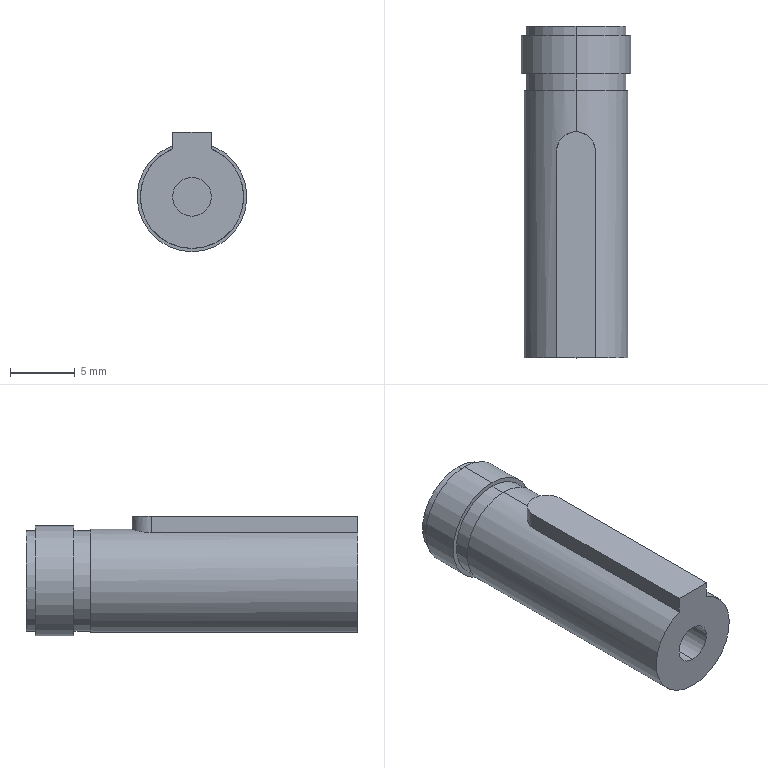Part | SolidWorks | features BaseBody 1 | 1 solid | 20 faces | box 8.5 x 25.7 x 9.25 mm | volume 1306 mm3 | cylinder 11 | plane 9 | commonest cylinder face diameters 7.8 x4 3 x3 8 x2 8.5 x2
STEP:
#1=CARTESIAN_POINT('',(0.,-10.31,-4.));
#2=VERTEX_POINT('',#1);
#3=CARTESIAN_POINT('',(0.,-10.31,4.));
#4=VERTEX_POINT('',#3);
#5=CARTESIAN_POINT('',(0.,-10.31,0.));
#6=DIRECTION('',(0.,-1.,0.));
#7=DIRECTION('',(0.,0.,-1.));
#8=AXIS2_PLACEMENT_3D('',#5,#6,#7);
#9=CIRCLE('',#8,4.);
#10=EDGE_CURVE('',#2,#4,#9,.T.);
#11=ORIENTED_EDGE('',*,*,#10,.T.);
#12=CARTESIAN_POINT('',(0.,-13.51,4.));
#13=VERTEX_POINT('',#12);
#14=CARTESIAN_POINT('',(0.,-20.66,4.));
#15=DIRECTION('',(0.,-1.,0.));
#16=VECTOR('',#15,1000.);
#17=LINE('',#14,#16);
#18=EDGE_CURVE('',#4,#13,#17,.T.);
#19=ORIENTED_EDGE('',*,*,#18,.T.);
#20=CARTESIAN_POINT('',(1.5,-15.01,3.708));
#21=VERTEX_POINT('',#20);
#22=CARTESIAN_POINT('',(0.,-13.51,4.));
#23=CARTESIAN_POINT('',(0.1,-13.51,4.));
#24=CARTESIAN_POINT('',(0.1982,-13.52,3.996));
#25=CARTESIAN_POINT('',(0.3911,-13.559,3.982));
#26=CARTESIAN_POINT('',(0.4868,-13.588,3.971));
#27=CARTESIAN_POINT('',(0.7587,-13.701,3.932));
#28=CARTESIAN_POINT('',(0.9238,-13.812,3.894));
#29=CARTESIAN_POINT('',(1.198,-14.086,3.819));
#30=CARTESIAN_POINT('',(1.309,-14.252,3.781));
#31=CARTESIAN_POINT('',(1.459,-14.612,3.725));
#32=CARTESIAN_POINT('',(1.5,-14.81,3.708));
#33=CARTESIAN_POINT('',(1.5,-15.01,3.708));
#34=B_SPLINE_CURVE_WITH_KNOTS('',3,(#22,#23,#24,#25,#26,#27,#28,#29,#30,#31,#32,#33),.UNSPECIFIED.,.F.,.F.,(4,2,2,2,2,4),(0.002365,0.002661,0.002956,0.003548,0.004139,0.00473),.UNSPECIFIED.);
#35=EDGE_CURVE('',#13,#21,#34,.T.);
#36=ORIENTED_EDGE('',*,*,#35,.T.);
#37=CARTESIAN_POINT('',(1.5,-31.01,3.708));
#38=VERTEX_POINT('',#37);
#39=CARTESIAN_POINT('',(1.5,-20.66,3.708));
#40=DIRECTION('',(0.,-1.,0.));
#41=VECTOR('',#40,1000.);
#42=LINE('',#39,#41);
#43=EDGE_CURVE('',#21,#38,#42,.T.);
#44=ORIENTED_EDGE('',*,*,#43,.T.);
#45=CARTESIAN_POINT('',(0.,-31.01,-4.));
#46=VERTEX_POINT('',#45);
#47=CARTESIAN_POINT('',(0.,-31.01,0.));
#48=DIRECTION('',(0.,1.,0.));
#49=DIRECTION('',(0.,0.,-1.));
#50=AXIS2_PLACEMENT_3D('',#47,#48,#49);
#51=CIRCLE('',#50,4.);
#52=EDGE_CURVE('',#38,#46,#51,.T.);
#53=ORIENTED_EDGE('',*,*,#52,.T.);
#54=CARTESIAN_POINT('',(0.,-20.66,-4.));
#55=DIRECTION('',(0.,-1.,0.));
#56=VECTOR('',#55,1000.);
#57=LINE('',#54,#56);
#58=EDGE_CURVE('',#2,#46,#57,.T.);
#59=ORIENTED_EDGE('',*,*,#58,.F.);
#60=EDGE_LOOP('',(#11,#19,#36,#44,#53,#59));
#61=FACE_OUTER_BOUND('',#60,.T.);
#62=CARTESIAN_POINT('',(0.,-20.66,0.));
#63=DIRECTION('',(0.,-1.,0.));
#64=DIRECTION('',(0.,0.,-1.));
#65=AXIS2_PLACEMENT_3D('',#62,#63,#64);
#66=CYLINDRICAL_SURFACE('',#65,4.);
#67=ADVANCED_FACE('',(#61),#66,.T.);
#68=CARTESIAN_POINT('',(0.,-23.01,1.5));
#69=VERTEX_POINT('',#68);
#70=CARTESIAN_POINT('',(0.,-23.01,-1.5));
#71=VERTEX_POINT('',#70);
#72=CARTESIAN_POINT('',(0.,-23.01,0.));
#73=DIRECTION('',(0.,-1.,0.));
#74=DIRECTION('',(0.,0.,-1.));
#75=AXIS2_PLACEMENT_3D('',#72,#73,#74);
#76=CIRCLE('',#75,1.5);
#77=EDGE_CURVE('',#69,#71,#76,.T.);
#78=ORIENTED_EDGE('',*,*,#77,.F.);
#79=CARTESIAN_POINT('',(0.,-31.01,1.5));
#80=VERTEX_POINT('',#79);
#81=CARTESIAN_POINT('',(0.,-27.01,1.5));
#82=DIRECTION('',(0.,-1.,0.));
#83=VECTOR('',#82,1000.);
#84=LINE('',#81,#83);
#85=EDGE_CURVE('',#69,#80,#84,.T.);
#86=ORIENTED_EDGE('',*,*,#85,.T.);
#87=CARTESIAN_POINT('',(0.,-31.01,-1.5));
#88=VERTEX_POINT('',#87);
#89=CARTESIAN_POINT('',(0.,-31.01,0.));
#90=DIRECTION('',(0.,1.,0.));
#91=DIRECTION('',(0.,0.,-1.));
#92=AXIS2_PLACEMENT_3D('',#89,#90,#91);
#93=CIRCLE('',#92,1.5);
#94=EDGE_CURVE('',#88,#80,#93,.T.);
#95=ORIENTED_EDGE('',*,*,#94,.F.);
#96=CARTESIAN_POINT('',(0.,-27.01,-1.5));
#97=DIRECTION('',(0.,-1.,0.));
#98=VECTOR('',#97,1000.);
#99=LINE('',#96,#98);
#100=EDGE_CURVE('',#71,#88,#99,.T.);
#101=ORIENTED_EDGE('',*,*,#100,.F.);
#102=EDGE_LOOP('',(#78,#86,#95,#101));
#103=FACE_OUTER_BOUND('',#102,.T.);
#104=CARTESIAN_POINT('',(0.,-27.01,0.));
#105=DIRECTION('',(0.,-1.,0.));
#106=DIRECTION('',(0.,0.,-1.));
#107=AXIS2_PLACEMENT_3D('',#104,#105,#106);
#108=CYLINDRICAL_SURFACE('',#107,1.5);
#109=ADVANCED_FACE('',(#103),#108,.F.);
#110=CARTESIAN_POINT('',(0.,-9.01,-3.9));
#111=VERTEX_POINT('',#110);
#112=CARTESIAN_POINT('',(0.,-9.01,3.9));
#113=VERTEX_POINT('',#112);
#114=CARTESIAN_POINT('',(0.,-9.01,0.));
#115=DIRECTION('',(0.,-1.,0.));
#116=DIRECTION('',(0.,0.,-1.));
#117=AXIS2_PLACEMENT_3D('',#114,#115,#116);
#118=CIRCLE('',#117,3.9);
#119=EDGE_CURVE('',#111,#113,#118,.T.);
#120=ORIENTED_EDGE('',*,*,#119,.T.);
#121=CARTESIAN_POINT('',(0.,-10.31,3.9));
#122=VERTEX_POINT('',#121);
#123=CARTESIAN_POINT('',(0.,-7.81,3.9));
#124=DIRECTION('',(0.,-1.,0.));
#125=VECTOR('',#124,1000.);
#126=LINE('',#123,#125);
#127=EDGE_CURVE('',#113,#122,#126,.T.);
#128=ORIENTED_EDGE('',*,*,#127,.T.);
#129=CARTESIAN_POINT('',(0.,-10.31,-3.9));
#130=VERTEX_POINT('',#129);
#131=CARTESIAN_POINT('',(0.,-10.31,0.));
#132=DIRECTION('',(0.,-1.,0.));
#133=DIRECTION('',(0.,0.,-1.));
#134=AXIS2_PLACEMENT_3D('',#131,#132,#133);
#135=CIRCLE('',#134,3.9);
#136=EDGE_CURVE('',#130,#122,#135,.T.);
#137=ORIENTED_EDGE('',*,*,#136,.F.);
#138=CARTESIAN_POINT('',(0.,-7.81,-3.9));
#139=DIRECTION('',(0.,-1.,0.));
#140=VECTOR('',#139,1000.);
#141=LINE('',#138,#140);
#142=EDGE_CURVE('',#111,#130,#141,.T.);
#143=ORIENTED_EDGE('',*,*,#142,.F.);
#144=EDGE_LOOP('',(#120,#128,#137,#143));
#145=FACE_OUTER_BOUND('',#144,.T.);
#146=CARTESIAN_POINT('',(0.,-7.81,0.));
#147=DIRECTION('',(0.,-1.,0.));
#148=DIRECTION('',(0.,0.,-1.));
#149=AXIS2_PLACEMENT_3D('',#146,#147,#148);
#150=CYLINDRICAL_SURFACE('',#149,3.9);
#151=ADVANCED_FACE('',(#145),#150,.T.);
#152=CARTESIAN_POINT('',(0.,-6.01,-4.25));
#153=VERTEX_POINT('',#152);
#154=CARTESIAN_POINT('',(0.,-6.01,4.25));
#155=VERTEX_POINT('',#154);
#156=CARTESIAN_POINT('',(0.,-6.01,0.));
#157=DIRECTION('',(0.,-1.,0.));
#158=DIRECTION('',(0.,0.,-1.));
#159=AXIS2_PLACEMENT_3D('',#156,#157,#158);
#160=CIRCLE('',#159,4.25);
#161=EDGE_CURVE('',#153,#155,#160,.T.);
#162=ORIENTED_EDGE('',*,*,#161,.T.);
#163=CARTESIAN_POINT('',(0.,-9.01,4.25));
#164=VERTEX_POINT('',#163);
#165=CARTESIAN_POINT('',(0.,-7.51,4.25));
#166=DIRECTION('',(0.,-1.,0.));
#167=VECTOR('',#166,1000.);
#168=LINE('',#165,#167);
#169=EDGE_CURVE('',#155,#164,#168,.T.);
#170=ORIENTED_EDGE('',*,*,#169,.T.);
#171=CARTESIAN_POINT('',(0.,-9.01,-4.25));
#172=VERTEX_POINT('',#171);
#173=CARTESIAN_POINT('',(0.,-9.01,0.));
#174=DIRECTION('',(0.,-1.,0.));
#175=DIRECTION('',(0.,0.,-1.));
#176=AXIS2_PLACEMENT_3D('',#173,#174,#175);
#177=CIRCLE('',#176,4.25);
#178=EDGE_CURVE('',#172,#164,#177,.T.);
#179=ORIENTED_EDGE('',*,*,#178,.F.);
#180=CARTESIAN_POINT('',(0.,-7.51,-4.25));
#181=DIRECTION('',(0.,-1.,0.));
#182=VECTOR('',#181,1000.);
#183=LINE('',#180,#182);
#184=EDGE_CURVE('',#153,#172,#183,.T.);
#185=ORIENTED_EDGE('',*,*,#184,.F.);
#186=EDGE_LOOP('',(#162,#170,#179,#185));
#187=FACE_OUTER_BOUND('',#186,.T.);
#188=CARTESIAN_POINT('',(0.,-7.51,0.));
#189=DIRECTION('',(0.,-1.,0.));
#190=DIRECTION('',(0.,0.,-1.));
#191=AXIS2_PLACEMENT_3D('',#188,#189,#190);
#192=CYLINDRICAL_SURFACE('',#191,4.25);
#193=ADVANCED_FACE('',(#187),#192,.T.);
#194=CARTESIAN_POINT('',(0.,-5.31,-3.9));
#195=VERTEX_POINT('',#194);
#196=CARTESIAN_POINT('',(0.,-5.31,3.9));
#197=VERTEX_POINT('',#196);
#198=CARTESIAN_POINT('',(0.,-5.31,0.));
#199=DIRECTION('',(0.,-1.,0.));
#200=DIRECTION('',(0.,0.,-1.));
#201=AXIS2_PLACEMENT_3D('',#198,#199,#200);
#202=CIRCLE('',#201,3.9);
#203=EDGE_CURVE('',#195,#197,#202,.T.);
#204=ORIENTED_EDGE('',*,*,#203,.T.);
#205=CARTESIAN_POINT('',(0.,-6.01,3.9));
#206=VERTEX_POINT('',#205);
#207=CARTESIAN_POINT('',(0.,-7.81,3.9));
#208=DIRECTION('',(0.,-1.,0.));
#209=VECTOR('',#208,1000.);
#210=LINE('',#207,#209);
#211=EDGE_CURVE('',#197,#206,#210,.T.);
#212=ORIENTED_EDGE('',*,*,#211,.T.);
#213=CARTESIAN_POINT('',(0.,-6.01,-3.9));
#214=VERTEX_POINT('',#213);
#215=CARTESIAN_POINT('',(0.,-6.01,0.));
#216=DIRECTION('',(0.,-1.,0.));
#217=DIRECTION('',(0.,0.,-1.));
#218=AXIS2_PLACEMENT_3D('',#215,#216,#217);
#219=CIRCLE('',#218,3.9);
#220=EDGE_CURVE('',#214,#206,#219,.T.);
#221=ORIENTED_EDGE('',*,*,#220,.F.);
#222=CARTESIAN_POINT('',(0.,-7.81,-3.9));
#223=DIRECTION('',(0.,-1.,0.));
#224=VECTOR('',#223,1000.);
#225=LINE('',#222,#224);
#226=EDGE_CURVE('',#195,#214,#225,.T.);
#227=ORIENTED_EDGE('',*,*,#226,.F.);
#228=EDGE_LOOP('',(#204,#212,#221,#227));
#229=FACE_OUTER_BOUND('',#228,.T.);
#230=CARTESIAN_POINT('',(0.,-7.81,0.));
#231=DIRECTION('',(0.,-1.,0.));
#232=DIRECTION('',(0.,0.,-1.));
#233=AXIS2_PLACEMENT_3D('',#230,#231,#232);
#234=CYLINDRICAL_SURFACE('',#233,3.9);
#235=ADVANCED_FACE('',(#229),#234,.T.);
#236=ORIENTED_EDGE('',*,*,#18,.F.);
#237=CARTESIAN_POINT('',(0.,-10.31,0.));
#238=DIRECTION('',(0.,-1.,0.));
#239=DIRECTION('',(0.,0.,-1.));
#240=AXIS2_PLACEMENT_3D('',#237,#238,#239);
#241=CIRCLE('',#240,4.);
#242=EDGE_CURVE('',#4,#2,#241,.T.);
#243=ORIENTED_EDGE('',*,*,#242,.T.);
#244=ORIENTED_EDGE('',*,*,#58,.T.);
#245=CARTESIAN_POINT('',(-1.5,-31.01,3.708));
#246=VERTEX_POINT('',#245);
#247=CARTESIAN_POINT('',(0.,-31.01,0.));
#248=DIRECTION('',(0.,1.,0.));
#249=DIRECTION('',(0.,0.,-1.));
#250=AXIS2_PLACEMENT_3D('',#247,#248,#249);
#251=CIRCLE('',#250,4.);
#252=EDGE_CURVE('',#46,#246,#251,.T.);
#253=ORIENTED_EDGE('',*,*,#252,.T.);
#254=CARTESIAN_POINT('',(-1.5,-15.01,3.708));
#255=VERTEX_POINT('',#254);
#256=CARTESIAN_POINT('',(-1.5,-20.66,3.708));
#257=DIRECTION('',(0.,1.,0.));
#258=VECTOR('',#257,1000.);
#259=LINE('',#256,#258);
#260=EDGE_CURVE('',#246,#255,#259,.T.);
#261=ORIENTED_EDGE('',*,*,#260,.T.);
#262=CARTESIAN_POINT('',(-1.5,-15.01,3.708));
#263=CARTESIAN_POINT('',(-1.5,-14.91,3.708));
#264=CARTESIAN_POINT('',(-1.49,-14.812,3.712));
#265=CARTESIAN_POINT('',(-1.451,-14.619,3.727));
#266=CARTESIAN_POINT('',(-1.422,-14.523,3.739));
#267=CARTESIAN_POINT('',(-1.309,-14.252,3.781));
#268=CARTESIAN_POINT('',(-1.198,-14.087,3.819));
#269=CARTESIAN_POINT('',(-0.9242,-13.813,3.894));
#270=CARTESIAN_POINT('',(-0.7585,-13.701,3.932));
#271=CARTESIAN_POINT('',(-0.3984,-13.551,3.984));
#272=CARTESIAN_POINT('',(-0.2001,-13.51,4.));
#273=CARTESIAN_POINT('',(0.,-13.51,4.));
#274=B_SPLINE_CURVE_WITH_KNOTS('',3,(#262,#263,#264,#265,#266,#267,#268,#269,#270,#271,#272,#273),.UNSPECIFIED.,.F.,.F.,(4,2,2,2,2,4),(0.,0.0002956,0.0005913,0.001183,0.001774,0.002365),.UNSPECIFIED.);
#275=EDGE_CURVE('',#255,#13,#274,.T.);
#276=ORIENTED_EDGE('',*,*,#275,.T.);
#277=EDGE_LOOP('',(#236,#243,#244,#253,#261,#276));
#278=FACE_OUTER_BOUND('',#277,.T.);
#279=CARTESIAN_POINT('',(0.,-20.66,0.));
#280=DIRECTION('',(0.,-1.,0.));
#281=DIRECTION('',(0.,0.,-1.));
#282=AXIS2_PLACEMENT_3D('',#279,#280,#281);
#283=CYLINDRICAL_SURFACE('',#282,4.);
#284=ADVANCED_FACE('',(#278),#283,.T.);
#285=CARTESIAN_POINT('',(-1.5,-15.01,5.));
#286=VERTEX_POINT('',#285);
#287=CARTESIAN_POINT('',(-1.5,-15.01,3.5));
#288=DIRECTION('',(0.,0.,1.));
#289=VECTOR('',#288,1000.);
#290=LINE('',#287,#289);
#291=EDGE_CURVE('',#255,#286,#290,.T.);
#292=ORIENTED_EDGE('',*,*,#291,.T.);
#293=CARTESIAN_POINT('',(1.5,-15.01,5.));
#294=VERTEX_POINT('',#293);
#295=CARTESIAN_POINT('',(0.,-15.01,5.));
#296=DIRECTION('',(0.,0.,-1.));
#297=DIRECTION('',(1.,0.,0.));
#298=AXIS2_PLACEMENT_3D('',#295,#296,#297);
#299=CIRCLE('',#298,1.5);
#300=EDGE_CURVE('',#286,#294,#299,.T.);
#301=ORIENTED_EDGE('',*,*,#300,.T.);
#302=CARTESIAN_POINT('',(1.5,-15.01,3.5));
#303=DIRECTION('',(0.,0.,-1.));
#304=VECTOR('',#303,1000.);
#305=LINE('',#302,#304);
#306=EDGE_CURVE('',#294,#21,#305,.T.);
#307=ORIENTED_EDGE('',*,*,#306,.T.);
#308=ORIENTED_EDGE('',*,*,#35,.F.);
#309=ORIENTED_EDGE('',*,*,#275,.F.);
#310=EDGE_LOOP('',(#292,#301,#307,#308,#309));
#311=FACE_OUTER_BOUND('',#310,.T.);
#312=CARTESIAN_POINT('',(0.,-15.01,3.5));
#313=DIRECTION('',(0.,0.,1.));
#314=DIRECTION('',(1.,0.,0.));
#315=AXIS2_PLACEMENT_3D('',#312,#313,#314);
#316=CYLINDRICAL_SURFACE('',#315,1.5);
#317=ADVANCED_FACE('',(#311),#316,.T.);
#318=CARTESIAN_POINT('',(-1.5,-31.01,5.));
#319=VERTEX_POINT('',#318);
#320=CARTESIAN_POINT('',(-1.5,-31.01,3.5));
#321=DIRECTION('',(0.,0.,-1.));
#322=VECTOR('',#321,1000.);
#323=LINE('',#320,#322);
#324=EDGE_CURVE('',#319,#246,#323,.T.);
#325=ORIENTED_EDGE('',*,*,#324,.F.);
#326=CARTESIAN_POINT('',(-1.5,-23.01,5.));
#327=DIRECTION('',(0.,-1.,0.));
#328=VECTOR('',#327,1000.);
#329=LINE('',#326,#328);
#330=EDGE_CURVE('',#286,#319,#329,.T.);
#331=ORIENTED_EDGE('',*,*,#330,.F.);
#332=ORIENTED_EDGE('',*,*,#291,.F.);
#333=ORIENTED_EDGE('',*,*,#260,.F.);
#334=EDGE_LOOP('',(#325,#331,#332,#333));
#335=FACE_OUTER_BOUND('',#334,.T.);
#336=CARTESIAN_POINT('',(-1.5,-23.01,3.5));
#337=DIRECTION('',(1.,0.,0.));
#338=DIRECTION('',(0.,0.,-1.));
#339=AXIS2_PLACEMENT_3D('',#336,#337,#338);
#340=PLANE('',#339);
#341=ADVANCED_FACE('',(#335),#340,.F.);
#342=ORIENTED_EDGE('',*,*,#94,.T.);
#343=CARTESIAN_POINT('',(0.,-31.01,0.));
#344=DIRECTION('',(0.,1.,0.));
#345=DIRECTION('',(0.,0.,-1.));
#346=AXIS2_PLACEMENT_3D('',#343,#344,#345);
#347=CIRCLE('',#346,1.5);
#348=EDGE_CURVE('',#80,#88,#347,.T.);
#349=ORIENTED_EDGE('',*,*,#348,.T.);
#350=EDGE_LOOP('',(#342,#349));
#351=FACE_BOUND('',#350,.T.);
#352=CARTESIAN_POINT('',(1.5,-31.01,5.));
#353=VERTEX_POINT('',#352);
#354=CARTESIAN_POINT('',(1.5,-31.01,3.5));
#355=DIRECTION('',(0.,0.,1.));
#356=VECTOR('',#355,1000.);
#357=LINE('',#354,#356);
#358=EDGE_CURVE('',#38,#353,#357,.T.);
#359=ORIENTED_EDGE('',*,*,#358,.T.);
#360=CARTESIAN_POINT('',(0.,-31.01,5.));
#361=DIRECTION('',(-1.,0.,0.));
#362=VECTOR('',#361,1000.);
#363=LINE('',#360,#362);
#364=EDGE_CURVE('',#353,#319,#363,.T.);
#365=ORIENTED_EDGE('',*,*,#364,.T.);
#366=ORIENTED_EDGE('',*,*,#324,.T.);
#367=ORIENTED_EDGE('',*,*,#252,.F.);
#368=ORIENTED_EDGE('',*,*,#52,.F.);
#369=EDGE_LOOP('',(#359,#365,#366,#367,#368));
#370=FACE_OUTER_BOUND('',#369,.T.);
#371=CARTESIAN_POINT('',(0.,-31.01,0.));
#372=DIRECTION('',(0.,-1.,0.));
#373=DIRECTION('',(0.,0.,-1.));
#374=AXIS2_PLACEMENT_3D('',#371,#372,#373);
#375=PLANE('',#374);
#376=ADVANCED_FACE('',(#351,#370),#375,.T.);
#377=ORIENTED_EDGE('',*,*,#136,.T.);
#378=CARTESIAN_POINT('',(0.,-10.31,0.));
#379=DIRECTION('',(0.,-1.,0.));
#380=DIRECTION('',(0.,0.,-1.));
#381=AXIS2_PLACEMENT_3D('',#378,#379,#380);
#382=CIRCLE('',#381,3.9);
#383=EDGE_CURVE('',#122,#130,#382,.T.);
#384=ORIENTED_EDGE('',*,*,#383,.T.);
#385=EDGE_LOOP('',(#377,#384));
#386=FACE_BOUND('',#385,.T.);
#387=ORIENTED_EDGE('',*,*,#10,.F.);
#388=ORIENTED_EDGE('',*,*,#242,.F.);
#389=EDGE_LOOP('',(#387,#388));
#390=FACE_OUTER_BOUND('',#389,.T.);
#391=CARTESIAN_POINT('',(0.,-10.31,0.));
#392=DIRECTION('',(0.,1.,0.));
#393=DIRECTION('',(0.,0.,1.));
#394=AXIS2_PLACEMENT_3D('',#391,#392,#393);
#395=PLANE('',#394);
#396=ADVANCED_FACE('',(#386,#390),#395,.T.);
#397=CARTESIAN_POINT('',(1.5,-23.01,5.));
#398=DIRECTION('',(0.,-1.,0.));
#399=VECTOR('',#398,1000.);
#400=LINE('',#397,#399);
#401=EDGE_CURVE('',#294,#353,#400,.T.);
#402=ORIENTED_EDGE('',*,*,#401,.F.);
#403=ORIENTED_EDGE('',*,*,#300,.F.);
#404=ORIENTED_EDGE('',*,*,#330,.T.);
#405=ORIENTED_EDGE('',*,*,#364,.F.);
#406=EDGE_LOOP('',(#402,#403,#404,#405));
#407=FACE_OUTER_BOUND('',#406,.T.);
#408=CARTESIAN_POINT('',(0.,-23.01,5.));
#409=DIRECTION('',(0.,0.,-1.));
#410=DIRECTION('',(-1.,0.,0.));
#411=AXIS2_PLACEMENT_3D('',#408,#409,#410);
#412=PLANE('',#411);
#413=ADVANCED_FACE('',(#407),#412,.F.);
#414=ORIENTED_EDGE('',*,*,#85,.F.);
#415=CARTESIAN_POINT('',(0.,-23.01,0.));
#416=DIRECTION('',(0.,-1.,0.));
#417=DIRECTION('',(0.,0.,-1.));
#418=AXIS2_PLACEMENT_3D('',#415,#416,#417);
#419=CIRCLE('',#418,1.5);
#420=EDGE_CURVE('',#71,#69,#419,.T.);
#421=ORIENTED_EDGE('',*,*,#420,.F.);
#422=ORIENTED_EDGE('',*,*,#100,.T.);
#423=ORIENTED_EDGE('',*,*,#348,.F.);
#424=EDGE_LOOP('',(#414,#421,#422,#423));
#425=FACE_OUTER_BOUND('',#424,.T.);
#426=CARTESIAN_POINT('',(0.,-27.01,0.));
#427=DIRECTION('',(0.,-1.,0.));
#428=DIRECTION('',(0.,0.,-1.));
#429=AXIS2_PLACEMENT_3D('',#426,#427,#428);
#430=CYLINDRICAL_SURFACE('',#429,1.5);
#431=ADVANCED_FACE('',(#425),#430,.F.);
#432=ORIENTED_EDGE('',*,*,#306,.F.);
#433=ORIENTED_EDGE('',*,*,#401,.T.);
#434=ORIENTED_EDGE('',*,*,#358,.F.);
#435=ORIENTED_EDGE('',*,*,#43,.F.);
#436=EDGE_LOOP('',(#432,#433,#434,#435));
#437=FACE_OUTER_BOUND('',#436,.T.);
#438=CARTESIAN_POINT('',(1.5,-23.01,3.5));
#439=DIRECTION('',(-1.,0.,0.));
#440=DIRECTION('',(0.,0.,1.));
#441=AXIS2_PLACEMENT_3D('',#438,#439,#440);
#442=PLANE('',#441);
#443=ADVANCED_FACE('',(#437),#442,.F.);
#444=ORIENTED_EDGE('',*,*,#127,.F.);
#445=CARTESIAN_POINT('',(0.,-9.01,0.));
#446=DIRECTION('',(0.,-1.,0.));
#447=DIRECTION('',(0.,0.,-1.));
#448=AXIS2_PLACEMENT_3D('',#445,#446,#447);
#449=CIRCLE('',#448,3.9);
#450=EDGE_CURVE('',#113,#111,#449,.T.);
#451=ORIENTED_EDGE('',*,*,#450,.T.);
#452=ORIENTED_EDGE('',*,*,#142,.T.);
#453=ORIENTED_EDGE('',*,*,#383,.F.);
#454=EDGE_LOOP('',(#444,#451,#452,#453));
#455=FACE_OUTER_BOUND('',#454,.T.);
#456=CARTESIAN_POINT('',(0.,-7.81,0.));
#457=DIRECTION('',(0.,-1.,0.));
#458=DIRECTION('',(0.,0.,-1.));
#459=AXIS2_PLACEMENT_3D('',#456,#457,#458);
#460=CYLINDRICAL_SURFACE('',#459,3.9);
#461=ADVANCED_FACE('',(#455),#460,.T.);
#462=ORIENTED_EDGE('',*,*,#420,.T.);
#463=ORIENTED_EDGE('',*,*,#77,.T.);
#464=EDGE_LOOP('',(#462,#463));
#465=FACE_OUTER_BOUND('',#464,.T.);
#466=CARTESIAN_POINT('',(0.,-23.01,0.));
#467=DIRECTION('',(0.,1.,0.));
#468=DIRECTION('',(0.,0.,1.));
#469=AXIS2_PLACEMENT_3D('',#466,#467,#468);
#470=PLANE('',#469);
#471=ADVANCED_FACE('',(#465),#470,.F.);
#472=ORIENTED_EDGE('',*,*,#178,.T.);
#473=CARTESIAN_POINT('',(0.,-9.01,0.));
#474=DIRECTION('',(0.,-1.,0.));
#475=DIRECTION('',(0.,0.,-1.));
#476=AXIS2_PLACEMENT_3D('',#473,#474,#475);
#477=CIRCLE('',#476,4.25);
#478=EDGE_CURVE('',#164,#172,#477,.T.);
#479=ORIENTED_EDGE('',*,*,#478,.T.);
#480=EDGE_LOOP('',(#472,#479));
#481=FACE_OUTER_BOUND('',#480,.T.);
#482=ORIENTED_EDGE('',*,*,#119,.F.);
#483=ORIENTED_EDGE('',*,*,#450,.F.);
#484=EDGE_LOOP('',(#482,#483));
#485=FACE_BOUND('',#484,.T.);
#486=CARTESIAN_POINT('',(0.,-9.01,0.));
#487=DIRECTION('',(0.,-1.,0.));
#488=DIRECTION('',(0.,0.,-1.));
#489=AXIS2_PLACEMENT_3D('',#486,#487,#488);
#490=PLANE('',#489);
#491=ADVANCED_FACE('',(#481,#485),#490,.T.);
#492=ORIENTED_EDGE('',*,*,#169,.F.);
#493=CARTESIAN_POINT('',(0.,-6.01,0.));
#494=DIRECTION('',(0.,-1.,0.));
#495=DIRECTION('',(0.,0.,-1.));
#496=AXIS2_PLACEMENT_3D('',#493,#494,#495);
#497=CIRCLE('',#496,4.25);
#498=EDGE_CURVE('',#155,#153,#497,.T.);
#499=ORIENTED_EDGE('',*,*,#498,.T.);
#500=ORIENTED_EDGE('',*,*,#184,.T.);
#501=ORIENTED_EDGE('',*,*,#478,.F.);
#502=EDGE_LOOP('',(#492,#499,#500,#501));
#503=FACE_OUTER_BOUND('',#502,.T.);
#504=CARTESIAN_POINT('',(0.,-7.51,0.));
#505=DIRECTION('',(0.,-1.,0.));
#506=DIRECTION('',(0.,0.,-1.));
#507=AXIS2_PLACEMENT_3D('',#504,#505,#506);
#508=CYLINDRICAL_SURFACE('',#507,4.25);
#509=ADVANCED_FACE('',(#503),#508,.T.);
#510=ORIENTED_EDGE('',*,*,#161,.F.);
#511=ORIENTED_EDGE('',*,*,#498,.F.);
#512=EDGE_LOOP('',(#510,#511));
#513=FACE_OUTER_BOUND('',#512,.T.);
#514=ORIENTED_EDGE('',*,*,#220,.T.);
#515=CARTESIAN_POINT('',(0.,-6.01,0.));
#516=DIRECTION('',(0.,-1.,0.));
#517=DIRECTION('',(0.,0.,-1.));
#518=AXIS2_PLACEMENT_3D('',#515,#516,#517);
#519=CIRCLE('',#518,3.9);
#520=EDGE_CURVE('',#206,#214,#519,.T.);
#521=ORIENTED_EDGE('',*,*,#520,.T.);
#522=EDGE_LOOP('',(#514,#521));
#523=FACE_BOUND('',#522,.T.);
#524=CARTESIAN_POINT('',(0.,-6.01,0.));
#525=DIRECTION('',(0.,1.,0.));
#526=DIRECTION('',(0.,0.,1.));
#527=AXIS2_PLACEMENT_3D('',#524,#525,#526);
#528=PLANE('',#527);
#529=ADVANCED_FACE('',(#513,#523),#528,.T.);
#530=ORIENTED_EDGE('',*,*,#211,.F.);
#531=CARTESIAN_POINT('',(0.,-5.31,0.));
#532=DIRECTION('',(0.,-1.,0.));
#533=DIRECTION('',(0.,0.,-1.));
#534=AXIS2_PLACEMENT_3D('',#531,#532,#533);
#535=CIRCLE('',#534,3.9);
#536=EDGE_CURVE('',#197,#195,#535,.T.);
#537=ORIENTED_EDGE('',*,*,#536,.T.);
#538=ORIENTED_EDGE('',*,*,#226,.T.);
#539=ORIENTED_EDGE('',*,*,#520,.F.);
#540=EDGE_LOOP('',(#530,#537,#538,#539));
#541=FACE_OUTER_BOUND('',#540,.T.);
#542=CARTESIAN_POINT('',(0.,-7.81,0.));
#543=DIRECTION('',(0.,-1.,0.));
#544=DIRECTION('',(0.,0.,-1.));
#545=AXIS2_PLACEMENT_3D('',#542,#543,#544);
#546=CYLINDRICAL_SURFACE('',#545,3.9);
#547=ADVANCED_FACE('',(#541),#546,.T.);
#548=ORIENTED_EDGE('',*,*,#203,.F.);
#549=ORIENTED_EDGE('',*,*,#536,.F.);
#550=EDGE_LOOP('',(#548,#549));
#551=FACE_OUTER_BOUND('',#550,.T.);
#552=CARTESIAN_POINT('',(0.,-5.31,0.));
#553=DIRECTION('',(0.,1.,0.));
#554=DIRECTION('',(0.,0.,1.));
#555=AXIS2_PLACEMENT_3D('',#552,#553,#554);
#556=PLANE('',#555);
#557=ADVANCED_FACE('',(#551),#556,.T.);
#558=CLOSED_SHELL('',(#67,#109,#151,#193,#235,#284,#317,#341,#376,#396,#413,#431,#443,#461,#471,#491,#509,#529,#547,#557));
#559=MANIFOLD_SOLID_BREP('',#558);
#560=CARTESIAN_POINT('',(0.,0.,0.));
#561=DIRECTION('',(0.,0.,1.));
#562=DIRECTION('',(1.,0.,0.));
#563=AXIS2_PLACEMENT_3D('',#560,#561,#562);
#564=(LENGTH_UNIT()NAMED_UNIT(*)SI_UNIT(.MILLI.,.METRE.));
#565=UNCERTAINTY_MEASURE_WITH_UNIT(LENGTH_MEASURE(0.00001),#564,'','');
#566=(NAMED_UNIT(*)PLANE_ANGLE_UNIT()SI_UNIT($,.RADIAN.));
#567=(NAMED_UNIT(*)SI_UNIT($,.STERADIAN.)SOLID_ANGLE_UNIT());
#568=(GEOMETRIC_REPRESENTATION_CONTEXT(3)GLOBAL_UNCERTAINTY_ASSIGNED_CONTEXT((#565))GLOBAL_UNIT_ASSIGNED_CONTEXT((#564,#566,#567))REPRESENTATION_CONTEXT('',''));
#569=ADVANCED_BREP_SHAPE_REPRESENTATION('',(#559,#563),#568);